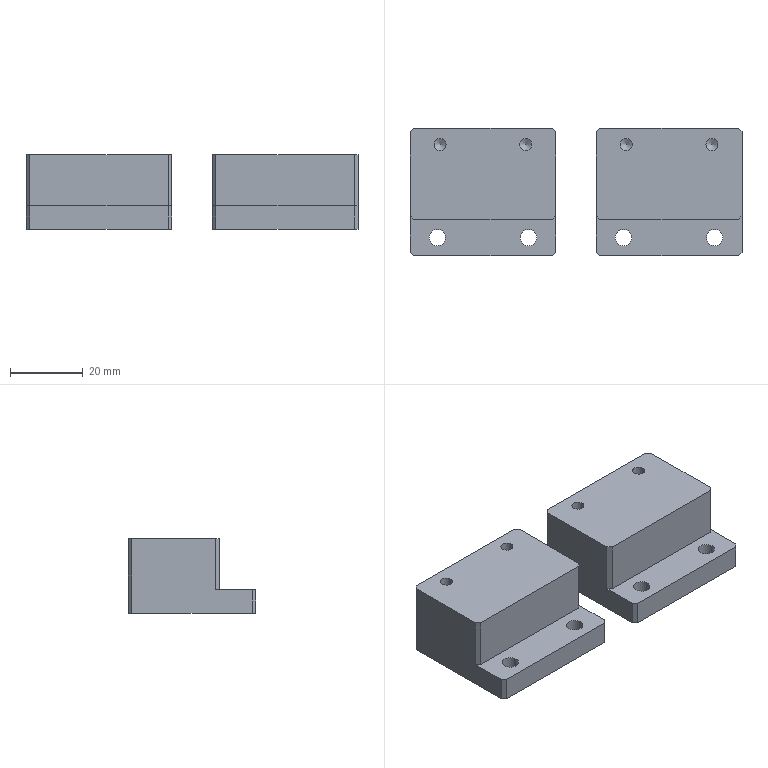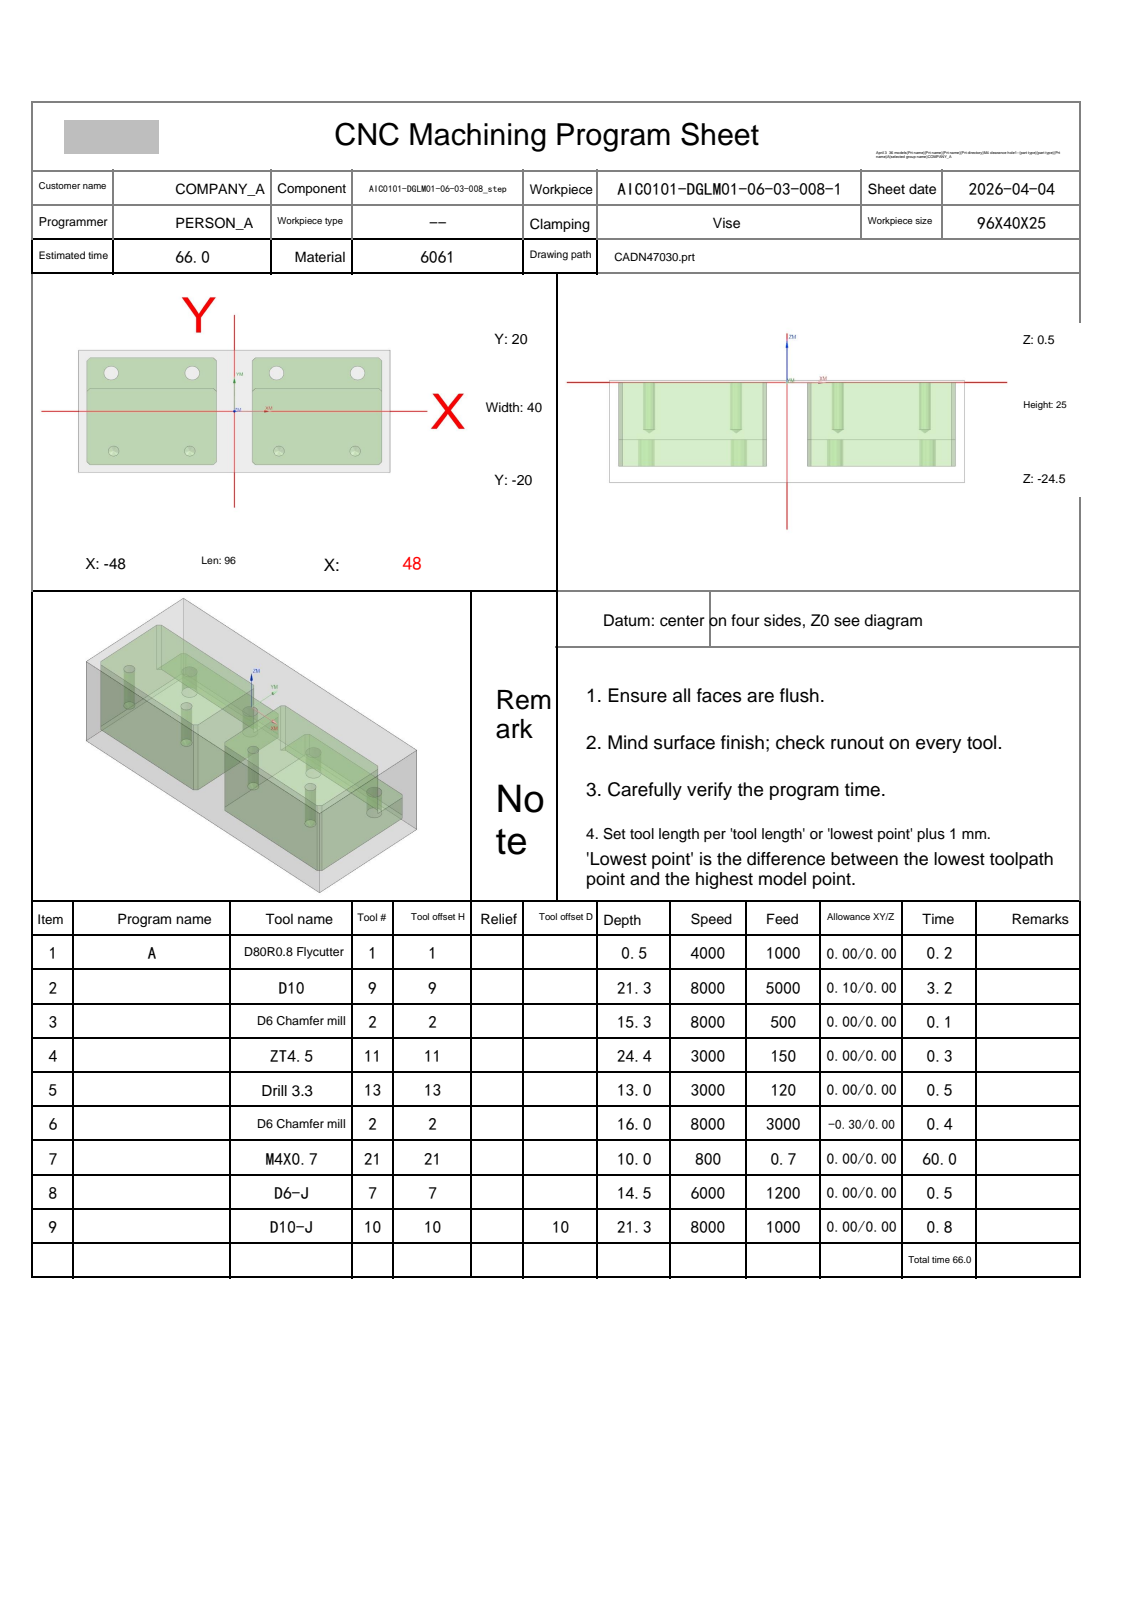NC program | NX | posted by the shop | part box 91 x 35 x 20.5 mm
Lines 2028 to 2147 of 2147:
N9 T10 M06
(D10-J  D=10. R=0. H=10 ce=0.00 di=0.00)
G00 G90 G54 X45.513 Y-23.616 M03 S8000
G43 H10 Z20.
M08
Z-9.9
G01 Z-10.4 F1000.
G41 D10
X45.497 Y-23.417
G03 X44.5 Y-22.5 I-.997 J-.083
G01 X6.5
G02 X2.964 Y-21.036 I0.0 J5.
G01 X1.964 Y-20.036
G02 X.5 Y-16.501 I3.536 J3.536
G01 Y16.501
G02 X1.964 Y20.036 I5. J-.001
G01 X2.964 Y21.036
G02 X6.5 Y22.5 I3.536 J-3.536
G01 X44.5
G02 X48.036 Y21.036 I0.0 J-5.
G01 X49.036 Y20.036
G02 X50.5 Y16.5 I-3.536 J-3.536
G01 Y-16.5
G02 X49.036 Y-20.036 I-5. J0.0
G01 X48.036 Y-21.036
G02 X44.5 Y-22.5 I-3.536 J3.536
G01 X44.
G03 X43. Y-23.5 I0.0 J-1.
G01 G40 Y-23.7
Z-9.9
G00 Z20.
X-24.5
Z-9.9
G01 Z-10.4
G41 D10
Y-23.5
G03 X-25.5 Y-22.5 I-1. J0.0
G01 X-44.5
G02 X-48.036 Y-21.036 I0.0 J5.
G01 X-49.036 Y-20.036
G02 X-50.5 Y-16.5 I3.536 J3.536
G01 Y16.5
G02 X-49.036 Y20.036 I5. J0.0
G01 X-48.036 Y21.036
G02 X-44.5 Y22.5 I3.536 J-3.536
G01 X-6.5
G02 X-2.964 Y21.036 I0.0 J-5.
G01 X-1.964 Y20.036
G02 X-.5 Y16.5 I-3.536 J-3.536
G01 Y-16.5
G02 X-1.964 Y-20.036 I-5. J0.0
G01 X-2.964 Y-21.036
G02 X-6.5 Y-22.5 I-3.536 J3.536
G01 X-25.5
X-26.
G03 X-27. Y-23.5 I0.0 J-1.
G01 G40 Y-23.7
Z-9.9
G00 Z20.
X45.513 Y-23.616
Z-20.3
G01 Z-20.8
G41 D10
X45.497 Y-23.417
G03 X44.5 Y-22.5 I-.997 J-.083
G01 X6.5
G02 X2.964 Y-21.036 I0.0 J5.
G01 X1.964 Y-20.036
G02 X.5 Y-16.5 I3.536 J3.536
G01 Y16.501
G02 X1.964 Y20.036 I5. J-.001
G01 X2.964 Y21.036
G02 X6.5 Y22.5 I3.536 J-3.536
G01 X44.5
G02 X48.036 Y21.036 I0.0 J-5.
G01 X49.036 Y20.036
G02 X50.5 Y16.5 I-3.536 J-3.536
G01 Y-16.5
G02 X49.036 Y-20.036 I-5. J0.0
G01 X48.036 Y-21.036
G02 X44.5 Y-22.5 I-3.536 J3.536
G01 X44.
G03 X43. Y-23.5 I0.0 J-1.
G01 G40 Y-23.7
Z-20.3
G00 Z20.
X-24.5
Z-20.3
G01 Z-20.8
G41 D10
Y-23.5
G03 X-25.5 Y-22.5 I-1. J0.0
G01 X-44.5
G02 X-48.036 Y-21.036 I0.0 J5.
G01 X-49.036 Y-20.036
G02 X-50.5 Y-16.5 I3.536 J3.536
G01 Y16.5
G02 X-49.036 Y20.036 I5. J0.0
G01 X-48.036 Y21.036
G02 X-44.5 Y22.5 I3.536 J-3.536
G01 X-6.5
G02 X-2.964 Y21.036 I0.0 J-5.
G01 X-1.964 Y20.036
G02 X-.5 Y16.5 I-3.536 J-3.536
G01 Y-16.5
G02 X-1.964 Y-20.036 I-5. J0.0
G01 X-2.964 Y-21.036
G02 X-6.5 Y-22.5 I-3.536 J3.536
G01 X-25.5
X-26.
G03 X-27. Y-23.5 I0.0 J-1.
G01 G40 Y-23.7
Z-20.3
G00 Z20.
M05
M09
G91 G28 Z0.0
G91 G28 Y0.0
M30
%